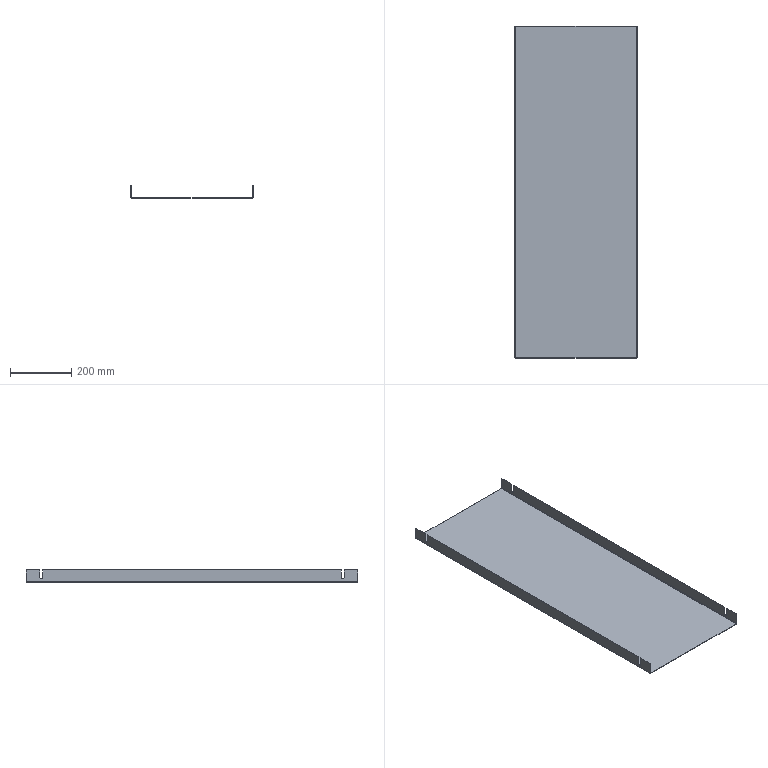Part | STEP file | 1.6米Belt线支撑(Default) | 1 solid | 42 faces | box 400 x 1085 x 40 mm | volume 772332 mm3 | plane 30 | cylinder 12 | commonest cylinder face diameters 9 x8 2 x2 5 x2
STEP:
#1=CARTESIAN_POINT('',(398.5,50.,-29.5));
#2=VERTEX_POINT('',#1);
#3=CARTESIAN_POINT('',(398.5,54.5,-25.));
#4=VERTEX_POINT('',#3);
#5=CARTESIAN_POINT('',(398.5,50.,-25.));
#6=DIRECTION('',(1.,0.,0.));
#7=DIRECTION('',(0.,0.,-1.));
#8=AXIS2_PLACEMENT_3D('',#5,#6,#7);
#9=CIRCLE('',#8,4.5);
#10=EDGE_CURVE('',#2,#4,#9,.T.);
#11=ORIENTED_EDGE('',*,*,#10,.F.);
#12=CARTESIAN_POINT('',(400.,50.,-29.5));
#13=VERTEX_POINT('',#12);
#14=CARTESIAN_POINT('',(0.,50.,-29.5));
#15=DIRECTION('',(1.,0.,0.));
#16=VECTOR('',#15,1000.);
#17=LINE('',#14,#16);
#18=EDGE_CURVE('',#2,#13,#17,.T.);
#19=ORIENTED_EDGE('',*,*,#18,.T.);
#20=CARTESIAN_POINT('',(400.,54.5,-25.));
#21=VERTEX_POINT('',#20);
#22=CARTESIAN_POINT('',(400.,50.,-25.));
#23=DIRECTION('',(1.,0.,0.));
#24=DIRECTION('',(0.,0.,-1.));
#25=AXIS2_PLACEMENT_3D('',#22,#23,#24);
#26=CIRCLE('',#25,4.5);
#27=EDGE_CURVE('',#13,#21,#26,.T.);
#28=ORIENTED_EDGE('',*,*,#27,.T.);
#29=CARTESIAN_POINT('',(0.,54.5,-25.));
#30=DIRECTION('',(1.,0.,0.));
#31=VECTOR('',#30,1000.);
#32=LINE('',#29,#31);
#33=EDGE_CURVE('',#4,#21,#32,.T.);
#34=ORIENTED_EDGE('',*,*,#33,.F.);
#35=EDGE_LOOP('',(#11,#19,#28,#34));
#36=FACE_OUTER_BOUND('',#35,.T.);
#37=CARTESIAN_POINT('',(0.,50.,-25.));
#38=DIRECTION('',(1.,0.,0.));
#39=DIRECTION('',(0.,0.,-1.));
#40=AXIS2_PLACEMENT_3D('',#37,#38,#39);
#41=CYLINDRICAL_SURFACE('',#40,4.5);
#42=ADVANCED_FACE('',(#36),#41,.F.);
#43=CARTESIAN_POINT('',(0.,50.,-29.5));
#44=VERTEX_POINT('',#43);
#45=CARTESIAN_POINT('',(0.,54.5,-25.));
#46=VERTEX_POINT('',#45);
#47=CARTESIAN_POINT('',(0.,50.,-25.));
#48=DIRECTION('',(1.,0.,0.));
#49=DIRECTION('',(0.,0.,-1.));
#50=AXIS2_PLACEMENT_3D('',#47,#48,#49);
#51=CIRCLE('',#50,4.5);
#52=EDGE_CURVE('',#44,#46,#51,.T.);
#53=ORIENTED_EDGE('',*,*,#52,.F.);
#54=CARTESIAN_POINT('',(1.5,50.,-29.5));
#55=VERTEX_POINT('',#54);
#56=CARTESIAN_POINT('',(0.,50.,-29.5));
#57=DIRECTION('',(1.,0.,0.));
#58=VECTOR('',#57,1000.);
#59=LINE('',#56,#58);
#60=EDGE_CURVE('',#44,#55,#59,.T.);
#61=ORIENTED_EDGE('',*,*,#60,.T.);
#62=CARTESIAN_POINT('',(1.5,54.5,-25.));
#63=VERTEX_POINT('',#62);
#64=CARTESIAN_POINT('',(1.5,50.,-25.));
#65=DIRECTION('',(-1.,0.,0.));
#66=DIRECTION('',(0.,0.,1.));
#67=AXIS2_PLACEMENT_3D('',#64,#65,#66);
#68=CIRCLE('',#67,4.5);
#69=EDGE_CURVE('',#63,#55,#68,.T.);
#70=ORIENTED_EDGE('',*,*,#69,.F.);
#71=CARTESIAN_POINT('',(0.,54.5,-25.));
#72=DIRECTION('',(1.,0.,0.));
#73=VECTOR('',#72,1000.);
#74=LINE('',#71,#73);
#75=EDGE_CURVE('',#46,#63,#74,.T.);
#76=ORIENTED_EDGE('',*,*,#75,.F.);
#77=EDGE_LOOP('',(#53,#61,#70,#76));
#78=FACE_OUTER_BOUND('',#77,.T.);
#79=CARTESIAN_POINT('',(0.,50.,-25.));
#80=DIRECTION('',(1.,0.,0.));
#81=DIRECTION('',(0.,0.,-1.));
#82=AXIS2_PLACEMENT_3D('',#79,#80,#81);
#83=CYLINDRICAL_SURFACE('',#82,4.5);
#84=ADVANCED_FACE('',(#78),#83,.F.);
#85=CARTESIAN_POINT('',(398.5,1035.,-29.5));
#86=VERTEX_POINT('',#85);
#87=CARTESIAN_POINT('',(398.5,1039.5,-25.));
#88=VERTEX_POINT('',#87);
#89=CARTESIAN_POINT('',(398.5,1035.,-25.));
#90=DIRECTION('',(1.,0.,0.));
#91=DIRECTION('',(0.,0.,-1.));
#92=AXIS2_PLACEMENT_3D('',#89,#90,#91);
#93=CIRCLE('',#92,4.5);
#94=EDGE_CURVE('',#86,#88,#93,.T.);
#95=ORIENTED_EDGE('',*,*,#94,.F.);
#96=CARTESIAN_POINT('',(400.,1035.,-29.5));
#97=VERTEX_POINT('',#96);
#98=CARTESIAN_POINT('',(0.,1035.,-29.5));
#99=DIRECTION('',(1.,0.,0.));
#100=VECTOR('',#99,1000.);
#101=LINE('',#98,#100);
#102=EDGE_CURVE('',#86,#97,#101,.T.);
#103=ORIENTED_EDGE('',*,*,#102,.T.);
#104=CARTESIAN_POINT('',(400.,1039.5,-25.));
#105=VERTEX_POINT('',#104);
#106=CARTESIAN_POINT('',(400.,1035.,-25.));
#107=DIRECTION('',(1.,0.,0.));
#108=DIRECTION('',(0.,0.,1.));
#109=AXIS2_PLACEMENT_3D('',#106,#107,#108);
#110=CIRCLE('',#109,4.5);
#111=EDGE_CURVE('',#97,#105,#110,.T.);
#112=ORIENTED_EDGE('',*,*,#111,.T.);
#113=CARTESIAN_POINT('',(0.,1039.5,-25.));
#114=DIRECTION('',(1.,0.,0.));
#115=VECTOR('',#114,1000.);
#116=LINE('',#113,#115);
#117=EDGE_CURVE('',#88,#105,#116,.T.);
#118=ORIENTED_EDGE('',*,*,#117,.F.);
#119=EDGE_LOOP('',(#95,#103,#112,#118));
#120=FACE_OUTER_BOUND('',#119,.T.);
#121=CARTESIAN_POINT('',(0.,1035.,-25.));
#122=DIRECTION('',(1.,0.,0.));
#123=DIRECTION('',(0.,0.,-1.));
#124=AXIS2_PLACEMENT_3D('',#121,#122,#123);
#125=CYLINDRICAL_SURFACE('',#124,4.5);
#126=ADVANCED_FACE('',(#120),#125,.F.);
#127=CARTESIAN_POINT('',(0.,1035.,-29.5));
#128=VERTEX_POINT('',#127);
#129=CARTESIAN_POINT('',(0.,1039.5,-25.));
#130=VERTEX_POINT('',#129);
#131=CARTESIAN_POINT('',(0.,1035.,-25.));
#132=DIRECTION('',(1.,0.,0.));
#133=DIRECTION('',(0.,0.,1.));
#134=AXIS2_PLACEMENT_3D('',#131,#132,#133);
#135=CIRCLE('',#134,4.5);
#136=EDGE_CURVE('',#128,#130,#135,.T.);
#137=ORIENTED_EDGE('',*,*,#136,.F.);
#138=CARTESIAN_POINT('',(1.5,1035.,-29.5));
#139=VERTEX_POINT('',#138);
#140=CARTESIAN_POINT('',(0.,1035.,-29.5));
#141=DIRECTION('',(1.,0.,0.));
#142=VECTOR('',#141,1000.);
#143=LINE('',#140,#142);
#144=EDGE_CURVE('',#128,#139,#143,.T.);
#145=ORIENTED_EDGE('',*,*,#144,.T.);
#146=CARTESIAN_POINT('',(1.5,1039.5,-25.));
#147=VERTEX_POINT('',#146);
#148=CARTESIAN_POINT('',(1.5,1035.,-25.));
#149=DIRECTION('',(-1.,0.,0.));
#150=DIRECTION('',(0.,0.,1.));
#151=AXIS2_PLACEMENT_3D('',#148,#149,#150);
#152=CIRCLE('',#151,4.5);
#153=EDGE_CURVE('',#147,#139,#152,.T.);
#154=ORIENTED_EDGE('',*,*,#153,.F.);
#155=CARTESIAN_POINT('',(0.,1039.5,-25.));
#156=DIRECTION('',(1.,0.,0.));
#157=VECTOR('',#156,1000.);
#158=LINE('',#155,#157);
#159=EDGE_CURVE('',#130,#147,#158,.T.);
#160=ORIENTED_EDGE('',*,*,#159,.F.);
#161=EDGE_LOOP('',(#137,#145,#154,#160));
#162=FACE_OUTER_BOUND('',#161,.T.);
#163=CARTESIAN_POINT('',(0.,1035.,-25.));
#164=DIRECTION('',(1.,0.,0.));
#165=DIRECTION('',(0.,0.,-1.));
#166=AXIS2_PLACEMENT_3D('',#163,#164,#165);
#167=CYLINDRICAL_SURFACE('',#166,4.5);
#168=ADVANCED_FACE('',(#162),#167,.F.);
#169=CARTESIAN_POINT('',(398.5,45.5,0.));
#170=VERTEX_POINT('',#169);
#171=CARTESIAN_POINT('',(400.,45.5,0.));
#172=VERTEX_POINT('',#171);
#173=CARTESIAN_POINT('',(400.,45.5,0.));
#174=DIRECTION('',(1.,0.,0.));
#175=VECTOR('',#174,1000.);
#176=LINE('',#173,#175);
#177=EDGE_CURVE('',#170,#172,#176,.T.);
#178=ORIENTED_EDGE('',*,*,#177,.F.);
#179=CARTESIAN_POINT('',(398.5,0.,0.));
#180=VERTEX_POINT('',#179);
#181=CARTESIAN_POINT('',(398.5,1085.,0.));
#182=DIRECTION('',(0.,-1.,0.));
#183=VECTOR('',#182,1000.);
#184=LINE('',#181,#183);
#185=EDGE_CURVE('',#170,#180,#184,.T.);
#186=ORIENTED_EDGE('',*,*,#185,.T.);
#187=CARTESIAN_POINT('',(400.,0.,0.));
#188=VERTEX_POINT('',#187);
#189=CARTESIAN_POINT('',(400.,0.,0.));
#190=DIRECTION('',(-1.,0.,0.));
#191=VECTOR('',#190,1000.);
#192=LINE('',#189,#191);
#193=EDGE_CURVE('',#188,#180,#192,.T.);
#194=ORIENTED_EDGE('',*,*,#193,.F.);
#195=CARTESIAN_POINT('',(400.,1085.,0.));
#196=DIRECTION('',(0.,-1.,0.));
#197=VECTOR('',#196,1000.);
#198=LINE('',#195,#197);
#199=EDGE_CURVE('',#172,#188,#198,.T.);
#200=ORIENTED_EDGE('',*,*,#199,.F.);
#201=EDGE_LOOP('',(#178,#186,#194,#200));
#202=FACE_OUTER_BOUND('',#201,.T.);
#203=CARTESIAN_POINT('',(400.,1085.,0.));
#204=DIRECTION('',(0.,0.,1.));
#205=DIRECTION('',(1.,0.,0.));
#206=AXIS2_PLACEMENT_3D('',#203,#204,#205);
#207=PLANE('',#206);
#208=ADVANCED_FACE('',(#202),#207,.T.);
#209=CARTESIAN_POINT('',(0.,45.5,0.));
#210=VERTEX_POINT('',#209);
#211=CARTESIAN_POINT('',(1.5,45.5,0.));
#212=VERTEX_POINT('',#211);
#213=CARTESIAN_POINT('',(1.5,45.5,0.));
#214=DIRECTION('',(1.,0.,0.));
#215=VECTOR('',#214,1000.);
#216=LINE('',#213,#215);
#217=EDGE_CURVE('',#210,#212,#216,.T.);
#218=ORIENTED_EDGE('',*,*,#217,.F.);
#219=CARTESIAN_POINT('',(0.,0.,0.));
#220=VERTEX_POINT('',#219);
#221=CARTESIAN_POINT('',(0.,1085.,0.));
#222=DIRECTION('',(0.,-1.,0.));
#223=VECTOR('',#222,1000.);
#224=LINE('',#221,#223);
#225=EDGE_CURVE('',#210,#220,#224,.T.);
#226=ORIENTED_EDGE('',*,*,#225,.T.);
#227=CARTESIAN_POINT('',(1.5,0.,0.));
#228=VERTEX_POINT('',#227);
#229=CARTESIAN_POINT('',(1.5,0.,0.));
#230=DIRECTION('',(-1.,0.,0.));
#231=VECTOR('',#230,1000.);
#232=LINE('',#229,#231);
#233=EDGE_CURVE('',#228,#220,#232,.T.);
#234=ORIENTED_EDGE('',*,*,#233,.F.);
#235=CARTESIAN_POINT('',(1.5,1085.,0.));
#236=DIRECTION('',(0.,-1.,0.));
#237=VECTOR('',#236,1000.);
#238=LINE('',#235,#237);
#239=EDGE_CURVE('',#212,#228,#238,.T.);
#240=ORIENTED_EDGE('',*,*,#239,.F.);
#241=EDGE_LOOP('',(#218,#226,#234,#240));
#242=FACE_OUTER_BOUND('',#241,.T.);
#243=CARTESIAN_POINT('',(1.5,1085.,0.));
#244=DIRECTION('',(0.,0.,1.));
#245=DIRECTION('',(1.,0.,0.));
#246=AXIS2_PLACEMENT_3D('',#243,#244,#245);
#247=PLANE('',#246);
#248=ADVANCED_FACE('',(#242),#247,.T.);
#249=CARTESIAN_POINT('',(400.,54.5,0.));
#250=VERTEX_POINT('',#249);
#251=CARTESIAN_POINT('',(398.5,54.5,0.));
#252=VERTEX_POINT('',#251);
#253=CARTESIAN_POINT('',(400.,54.5,0.));
#254=DIRECTION('',(-1.,0.,0.));
#255=VECTOR('',#254,1000.);
#256=LINE('',#253,#255);
#257=EDGE_CURVE('',#250,#252,#256,.T.);
#258=ORIENTED_EDGE('',*,*,#257,.F.);
#259=CARTESIAN_POINT('',(400.,1030.5,0.));
#260=VERTEX_POINT('',#259);
#261=CARTESIAN_POINT('',(400.,1085.,0.));
#262=DIRECTION('',(0.,-1.,0.));
#263=VECTOR('',#262,1000.);
#264=LINE('',#261,#263);
#265=EDGE_CURVE('',#260,#250,#264,.T.);
#266=ORIENTED_EDGE('',*,*,#265,.F.);
#267=CARTESIAN_POINT('',(398.5,1030.5,0.));
#268=VERTEX_POINT('',#267);
#269=CARTESIAN_POINT('',(400.,1030.5,0.));
#270=DIRECTION('',(1.,0.,0.));
#271=VECTOR('',#270,1000.);
#272=LINE('',#269,#271);
#273=EDGE_CURVE('',#268,#260,#272,.T.);
#274=ORIENTED_EDGE('',*,*,#273,.F.);
#275=CARTESIAN_POINT('',(398.5,1085.,0.));
#276=DIRECTION('',(0.,-1.,0.));
#277=VECTOR('',#276,1000.);
#278=LINE('',#275,#277);
#279=EDGE_CURVE('',#268,#252,#278,.T.);
#280=ORIENTED_EDGE('',*,*,#279,.T.);
#281=EDGE_LOOP('',(#258,#266,#274,#280));
#282=FACE_OUTER_BOUND('',#281,.T.);
#283=CARTESIAN_POINT('',(400.,1085.,0.));
#284=DIRECTION('',(0.,0.,1.));
#285=DIRECTION('',(1.,0.,0.));
#286=AXIS2_PLACEMENT_3D('',#283,#284,#285);
#287=PLANE('',#286);
#288=ADVANCED_FACE('',(#282),#287,.T.);
#289=CARTESIAN_POINT('',(1.5,54.5,0.));
#290=VERTEX_POINT('',#289);
#291=CARTESIAN_POINT('',(0.,54.5,0.));
#292=VERTEX_POINT('',#291);
#293=CARTESIAN_POINT('',(1.5,54.5,0.));
#294=DIRECTION('',(-1.,0.,0.));
#295=VECTOR('',#294,1000.);
#296=LINE('',#293,#295);
#297=EDGE_CURVE('',#290,#292,#296,.T.);
#298=ORIENTED_EDGE('',*,*,#297,.F.);
#299=CARTESIAN_POINT('',(1.5,1030.5,0.));
#300=VERTEX_POINT('',#299);
#301=CARTESIAN_POINT('',(1.5,1085.,0.));
#302=DIRECTION('',(0.,-1.,0.));
#303=VECTOR('',#302,1000.);
#304=LINE('',#301,#303);
#305=EDGE_CURVE('',#300,#290,#304,.T.);
#306=ORIENTED_EDGE('',*,*,#305,.F.);
#307=CARTESIAN_POINT('',(0.,1030.5,0.));
#308=VERTEX_POINT('',#307);
#309=CARTESIAN_POINT('',(1.5,1030.5,0.));
#310=DIRECTION('',(1.,0.,0.));
#311=VECTOR('',#310,1000.);
#312=LINE('',#309,#311);
#313=EDGE_CURVE('',#308,#300,#312,.T.);
#314=ORIENTED_EDGE('',*,*,#313,.F.);
#315=CARTESIAN_POINT('',(0.,1085.,0.));
#316=DIRECTION('',(0.,-1.,0.));
#317=VECTOR('',#316,1000.);
#318=LINE('',#315,#317);
#319=EDGE_CURVE('',#308,#292,#318,.T.);
#320=ORIENTED_EDGE('',*,*,#319,.T.);
#321=EDGE_LOOP('',(#298,#306,#314,#320));
#322=FACE_OUTER_BOUND('',#321,.T.);
#323=CARTESIAN_POINT('',(1.5,1085.,0.));
#324=DIRECTION('',(0.,0.,1.));
#325=DIRECTION('',(1.,0.,0.));
#326=AXIS2_PLACEMENT_3D('',#323,#324,#325);
#327=PLANE('',#326);
#328=ADVANCED_FACE('',(#322),#327,.T.);
#329=CARTESIAN_POINT('',(2.5,1085.,-40.));
#330=VERTEX_POINT('',#329);
#331=CARTESIAN_POINT('',(2.5,1085.,-38.5));
#332=VERTEX_POINT('',#331);
#333=CARTESIAN_POINT('',(2.5,1085.,-40.));
#334=DIRECTION('',(0.,0.,1.));
#335=VECTOR('',#334,1000.);
#336=LINE('',#333,#335);
#337=EDGE_CURVE('',#330,#332,#336,.T.);
#338=ORIENTED_EDGE('',*,*,#337,.F.);
#339=CARTESIAN_POINT('',(0.,1085.,-37.5));
#340=VERTEX_POINT('',#339);
#341=CARTESIAN_POINT('',(2.5,1085.,-37.5));
#342=DIRECTION('',(0.,-1.,0.));
#343=DIRECTION('',(0.,0.,1.));
#344=AXIS2_PLACEMENT_3D('',#341,#342,#343);
#345=CIRCLE('',#344,2.5);
#346=EDGE_CURVE('',#340,#330,#345,.T.);
#347=ORIENTED_EDGE('',*,*,#346,.F.);
#348=CARTESIAN_POINT('',(1.5,1085.,-37.5));
#349=VERTEX_POINT('',#348);
#350=CARTESIAN_POINT('',(1.5,1085.,-37.5));
#351=DIRECTION('',(-1.,0.,0.));
#352=VECTOR('',#351,1000.);
#353=LINE('',#350,#352);
#354=EDGE_CURVE('',#349,#340,#353,.T.);
#355=ORIENTED_EDGE('',*,*,#354,.F.);
#356=CARTESIAN_POINT('',(2.5,1085.,-37.5));
#357=DIRECTION('',(0.,-1.,0.));
#358=DIRECTION('',(1.,0.,0.));
#359=AXIS2_PLACEMENT_3D('',#356,#357,#358);
#360=CIRCLE('',#359,1.);
#361=EDGE_CURVE('',#349,#332,#360,.T.);
#362=ORIENTED_EDGE('',*,*,#361,.T.);
#363=EDGE_LOOP('',(#338,#347,#355,#362));
#364=FACE_OUTER_BOUND('',#363,.T.);
#365=CARTESIAN_POINT('',(2.5,1085.,-40.));
#366=DIRECTION('',(0.,1.,0.));
#367=DIRECTION('',(0.,0.,1.));
#368=AXIS2_PLACEMENT_3D('',#365,#366,#367);
#369=PLANE('',#368);
#370=ADVANCED_FACE('',(#364),#369,.T.);
#371=CARTESIAN_POINT('',(397.5,1085.,-40.));
#372=VERTEX_POINT('',#371);
#373=CARTESIAN_POINT('',(0.,1085.,-40.));
#374=DIRECTION('',(1.,0.,0.));
#375=VECTOR('',#374,1000.);
#376=LINE('',#373,#375);
#377=EDGE_CURVE('',#330,#372,#376,.T.);
#378=ORIENTED_EDGE('',*,*,#377,.F.);
#379=ORIENTED_EDGE('',*,*,#337,.T.);
#380=CARTESIAN_POINT('',(397.5,1085.,-38.5));
#381=VERTEX_POINT('',#380);
#382=CARTESIAN_POINT('',(0.,1085.,-38.5));
#383=DIRECTION('',(1.,0.,0.));
#384=VECTOR('',#383,1000.);
#385=LINE('',#382,#384);
#386=EDGE_CURVE('',#332,#381,#385,.T.);
#387=ORIENTED_EDGE('',*,*,#386,.T.);
#388=CARTESIAN_POINT('',(397.5,1085.,-38.5));
#389=DIRECTION('',(0.,0.,-1.));
#390=VECTOR('',#389,1000.);
#391=LINE('',#388,#390);
#392=EDGE_CURVE('',#381,#372,#391,.T.);
#393=ORIENTED_EDGE('',*,*,#392,.T.);
#394=EDGE_LOOP('',(#378,#379,#387,#393));
#395=FACE_OUTER_BOUND('',#394,.T.);
#396=CARTESIAN_POINT('',(1.5,1085.,-37.5));
#397=DIRECTION('',(0.,1.,0.));
#398=DIRECTION('',(0.,0.,1.));
#399=AXIS2_PLACEMENT_3D('',#396,#397,#398);
#400=PLANE('',#399);
#401=ADVANCED_FACE('',(#395),#400,.T.);
#402=CARTESIAN_POINT('',(0.,0.,-37.5));
#403=VERTEX_POINT('',#402);
#404=CARTESIAN_POINT('',(1.5,0.,-37.5));
#405=VERTEX_POINT('',#404);
#406=CARTESIAN_POINT('',(0.,0.,-37.5));
#407=DIRECTION('',(1.,0.,0.));
#408=VECTOR('',#407,1000.);
#409=LINE('',#406,#408);
#410=EDGE_CURVE('',#403,#405,#409,.T.);
#411=ORIENTED_EDGE('',*,*,#410,.F.);
#412=CARTESIAN_POINT('',(2.5,0.,-40.));
#413=VERTEX_POINT('',#412);
#414=CARTESIAN_POINT('',(2.5,0.,-37.5));
#415=DIRECTION('',(0.,-1.,0.));
#416=DIRECTION('',(0.,0.,1.));
#417=AXIS2_PLACEMENT_3D('',#414,#415,#416);
#418=CIRCLE('',#417,2.5);
#419=EDGE_CURVE('',#403,#413,#418,.T.);
#420=ORIENTED_EDGE('',*,*,#419,.T.);
#421=CARTESIAN_POINT('',(2.5,0.,-38.5));
#422=VERTEX_POINT('',#421);
#423=CARTESIAN_POINT('',(2.5,0.,-38.5));
#424=DIRECTION('',(0.,0.,-1.));
#425=VECTOR('',#424,1000.);
#426=LINE('',#423,#425);
#427=EDGE_CURVE('',#422,#413,#426,.T.);
#428=ORIENTED_EDGE('',*,*,#427,.F.);
#429=CARTESIAN_POINT('',(2.5,0.,-37.5));
#430=DIRECTION('',(0.,-1.,0.));
#431=DIRECTION('',(1.,0.,0.));
#432=AXIS2_PLACEMENT_3D('',#429,#430,#431);
#433=CIRCLE('',#432,1.);
#434=EDGE_CURVE('',#405,#422,#433,.T.);
#435=ORIENTED_EDGE('',*,*,#434,.F.);
#436=EDGE_LOOP('',(#411,#420,#428,#435));
#437=FACE_OUTER_BOUND('',#436,.T.);
#438=CARTESIAN_POINT('',(0.,0.,-37.5));
#439=DIRECTION('',(0.,-1.,0.));
#440=DIRECTION('',(0.,0.,-1.));
#441=AXIS2_PLACEMENT_3D('',#438,#439,#440);
#442=PLANE('',#441);
#443=ADVANCED_FACE('',(#437),#442,.T.);
#444=CARTESIAN_POINT('',(0.,0.,0.));
#445=DIRECTION('',(0.,0.,-1.));
#446=VECTOR('',#445,1000.);
#447=LINE('',#444,#446);
#448=EDGE_CURVE('',#220,#403,#447,.T.);
#449=ORIENTED_EDGE('',*,*,#448,.T.);
#450=ORIENTED_EDGE('',*,*,#410,.T.);
#451=CARTESIAN_POINT('',(1.5,0.,0.));
#452=DIRECTION('',(0.,0.,-1.));
#453=VECTOR('',#452,1000.);
#454=LINE('',#451,#453);
#455=EDGE_CURVE('',#228,#405,#454,.T.);
#456=ORIENTED_EDGE('',*,*,#455,.F.);
#457=ORIENTED_EDGE('',*,*,#233,.T.);
#458=EDGE_LOOP('',(#449,#450,#456,#457));
#459=FACE_OUTER_BOUND('',#458,.T.);
#460=CARTESIAN_POINT('',(2.5,0.,-38.5));
#461=DIRECTION('',(0.,-1.,0.));
#462=DIRECTION('',(0.,0.,-1.));
#463=AXIS2_PLACEMENT_3D('',#460,#461,#462);
#464=PLANE('',#463);
#465=ADVANCED_FACE('',(#459),#464,.T.);
#466=CARTESIAN_POINT('',(400.,1085.,-37.5));
#467=VERTEX_POINT('',#466);
#468=CARTESIAN_POINT('',(398.5,1085.,-37.5));
#469=VERTEX_POINT('',#468);
#470=CARTESIAN_POINT('',(400.,1085.,-37.5));
#471=DIRECTION('',(-1.,0.,0.));
#472=VECTOR('',#471,1000.);
#473=LINE('',#470,#472);
#474=EDGE_CURVE('',#467,#469,#473,.T.);
#475=ORIENTED_EDGE('',*,*,#474,.F.);
#476=CARTESIAN_POINT('',(397.5,1085.,-37.5));
#477=DIRECTION('',(0.,-1.,0.));
#478=DIRECTION('',(0.,0.,1.));
#479=AXIS2_PLACEMENT_3D('',#476,#477,#478);
#480=CIRCLE('',#479,2.5);
#481=EDGE_CURVE('',#372,#467,#480,.T.);
#482=ORIENTED_EDGE('',*,*,#481,.F.);
#483=ORIENTED_EDGE('',*,*,#392,.F.);
#484=CARTESIAN_POINT('',(397.5,1085.,-37.5));
#485=DIRECTION('',(0.,-1.,0.));
#486=DIRECTION('',(1.,0.,0.));
#487=AXIS2_PLACEMENT_3D('',#484,#485,#486);
#488=CIRCLE('',#487,1.);
#489=EDGE_CURVE('',#381,#469,#488,.T.);
#490=ORIENTED_EDGE('',*,*,#489,.T.);
#491=EDGE_LOOP('',(#475,#482,#483,#490));
#492=FACE_OUTER_BOUND('',#491,.T.);
#493=CARTESIAN_POINT('',(400.,1085.,-37.5));
#494=DIRECTION('',(0.,1.,0.));
#495=DIRECTION('',(0.,0.,1.));
#496=AXIS2_PLACEMENT_3D('',#493,#494,#495);
#497=PLANE('',#496);
#498=ADVANCED_FACE('',(#492),#497,.T.);
#499=CARTESIAN_POINT('',(400.,1085.,0.));
#500=VERTEX_POINT('',#499);
#501=CARTESIAN_POINT('',(400.,1085.,-40.));
#502=DIRECTION('',(0.,0.,1.));
#503=VECTOR('',#502,1000.);
#504=LINE('',#501,#503);
#505=EDGE_CURVE('',#467,#500,#504,.T.);
#506=ORIENTED_EDGE('',*,*,#505,.F.);
#507=ORIENTED_EDGE('',*,*,#474,.T.);
#508=CARTESIAN_POINT('',(398.5,1085.,0.));
#509=VERTEX_POINT('',#508);
#510=CARTESIAN_POINT('',(398.5,1085.,-40.));
#511=DIRECTION('',(0.,0.,1.));
#512=VECTOR('',#511,1000.);
#513=LINE('',#510,#512);
#514=EDGE_CURVE('',#469,#509,#513,.T.);
#515=ORIENTED_EDGE('',*,*,#514,.T.);
#516=CARTESIAN_POINT('',(400.,1085.,0.));
#517=DIRECTION('',(-1.,0.,0.));
#518=VECTOR('',#517,1000.);
#519=LINE('',#516,#518);
#520=EDGE_CURVE('',#500,#509,#519,.T.);
#521=ORIENTED_EDGE('',*,*,#520,.F.);
#522=EDGE_LOOP('',(#506,#507,#515,#521));
#523=FACE_OUTER_BOUND('',#522,.T.);
#524=CARTESIAN_POINT('',(397.5,1085.,-38.5));
#525=DIRECTION('',(0.,1.,0.));
#526=DIRECTION('',(0.,0.,1.));
#527=AXIS2_PLACEMENT_3D('',#524,#525,#526);
#528=PLANE('',#527);
#529=ADVANCED_FACE('',(#523),#528,.T.);
#530=CARTESIAN_POINT('',(397.5,0.,-40.));
#531=VERTEX_POINT('',#530);
#532=CARTESIAN_POINT('',(397.5,0.,-38.5));
#533=VERTEX_POINT('',#532);
#534=CARTESIAN_POINT('',(397.5,0.,-40.));
#535=DIRECTION('',(0.,0.,1.));
#536=VECTOR('',#535,1000.);
#537=LINE('',#534,#536);
#538=EDGE_CURVE('',#531,#533,#537,.T.);
#539=ORIENTED_EDGE('',*,*,#538,.F.);
#540=CARTESIAN_POINT('',(400.,0.,-37.5));
#541=VERTEX_POINT('',#540);
#542=CARTESIAN_POINT('',(397.5,0.,-37.5));
#543=DIRECTION('',(0.,-1.,0.));
#544=DIRECTION('',(0.,0.,1.));
#545=AXIS2_PLACEMENT_3D('',#542,#543,#544);
#546=CIRCLE('',#545,2.5);
#547=EDGE_CURVE('',#531,#541,#546,.T.);
#548=ORIENTED_EDGE('',*,*,#547,.T.);
#549=CARTESIAN_POINT('',(398.5,0.,-37.5));
#550=VERTEX_POINT('',#549);
#551=CARTESIAN_POINT('',(398.5,0.,-37.5));
#552=DIRECTION('',(1.,0.,0.));
#553=VECTOR('',#552,1000.);
#554=LINE('',#551,#553);
#555=EDGE_CURVE('',#550,#541,#554,.T.);
#556=ORIENTED_EDGE('',*,*,#555,.F.);
#557=CARTESIAN_POINT('',(397.5,0.,-37.5));
#558=DIRECTION('',(0.,-1.,0.));
#559=DIRECTION('',(1.,0.,0.));
#560=AXIS2_PLACEMENT_3D('',#557,#558,#559);
#561=CIRCLE('',#560,1.);
#562=EDGE_CURVE('',#533,#550,#561,.T.);
#563=ORIENTED_EDGE('',*,*,#562,.F.);
#564=EDGE_LOOP('',(#539,#548,#556,#563));
#565=FACE_OUTER_BOUND('',#564,.T.);
#566=CARTESIAN_POINT('',(397.5,0.,-40.));
#567=DIRECTION('',(0.,-1.,0.));
#568=DIRECTION('',(0.,0.,-1.));
#569=AXIS2_PLACEMENT_3D('',#566,#567,#568);
#570=PLANE('',#569);
#571=ADVANCED_FACE('',(#565),#570,.T.);
#572=CARTESIAN_POINT('',(0.,0.,-40.));
#573=DIRECTION('',(1.,0.,0.));
#574=VECTOR('',#573,1000.);
#575=LINE('',#572,#574);
#576=EDGE_CURVE('',#413,#531,#575,.T.);
#577=ORIENTED_EDGE('',*,*,#576,.T.);
#578=ORIENTED_EDGE('',*,*,#538,.T.);
#579=CARTESIAN_POINT('',(0.,0.,-38.5));
#580=DIRECTION('',(1.,0.,0.));
#581=VECTOR('',#580,1000.);
#582=LINE('',#579,#581);
#583=EDGE_CURVE('',#422,#533,#582,.T.);
#584=ORIENTED_EDGE('',*,*,#583,.F.);
#585=ORIENTED_EDGE('',*,*,#427,.T.);
#586=EDGE_LOOP('',(#577,#578,#584,#585));
#587=FACE_OUTER_BOUND('',#586,.T.);
#588=CARTESIAN_POINT('',(398.5,0.,-37.5));
#589=DIRECTION('',(0.,-1.,0.));
#590=DIRECTION('',(0.,0.,-1.));
#591=AXIS2_PLACEMENT_3D('',#588,#589,#590);
#592=PLANE('',#591);
#593=ADVANCED_FACE('',(#587),#592,.T.);
#594=ORIENTED_EDGE('',*,*,#185,.F.);
#595=CARTESIAN_POINT('',(398.5,45.5,-25.));
#596=VERTEX_POINT('',#595);
#597=CARTESIAN_POINT('',(398.5,45.5,-40.));
#598=DIRECTION('',(0.,0.,-1.));
#599=VECTOR('',#598,1000.);
#600=LINE('',#597,#599);
#601=EDGE_CURVE('',#170,#596,#600,.T.);
#602=ORIENTED_EDGE('',*,*,#601,.T.);
#603=CARTESIAN_POINT('',(398.5,50.,-25.));
#604=DIRECTION('',(1.,0.,0.));
#605=DIRECTION('',(0.,0.,-1.));
#606=AXIS2_PLACEMENT_3D('',#603,#604,#605);
#607=CIRCLE('',#606,4.5);
#608=EDGE_CURVE('',#596,#2,#607,.T.);
#609=ORIENTED_EDGE('',*,*,#608,.T.);
#610=ORIENTED_EDGE('',*,*,#10,.T.);
#611=CARTESIAN_POINT('',(398.5,54.5,-40.));
#612=DIRECTION('',(0.,0.,1.));
#613=VECTOR('',#612,1000.);
#614=LINE('',#611,#613);
#615=EDGE_CURVE('',#4,#252,#614,.T.);
#616=ORIENTED_EDGE('',*,*,#615,.T.);
#617=ORIENTED_EDGE('',*,*,#279,.F.);
#618=CARTESIAN_POINT('',(398.5,1030.5,-25.));
#619=VERTEX_POINT('',#618);
#620=CARTESIAN_POINT('',(398.5,1030.5,-40.));
#621=DIRECTION('',(0.,0.,-1.));
#622=VECTOR('',#621,1000.);
#623=LINE('',#620,#622);
#624=EDGE_CURVE('',#268,#619,#623,.T.);
#625=ORIENTED_EDGE('',*,*,#624,.T.);
#626=CARTESIAN_POINT('',(398.5,1035.,-25.));
#627=DIRECTION('',(1.,0.,0.));
#628=DIRECTION('',(0.,0.,-1.));
#629=AXIS2_PLACEMENT_3D('',#626,#627,#628);
#630=CIRCLE('',#629,4.5);
#631=EDGE_CURVE('',#619,#86,#630,.T.);
#632=ORIENTED_EDGE('',*,*,#631,.T.);
#633=ORIENTED_EDGE('',*,*,#94,.T.);
#634=CARTESIAN_POINT('',(398.5,1039.5,0.));
#635=VERTEX_POINT('',#634);
#636=CARTESIAN_POINT('',(398.5,1039.5,-40.));
#637=DIRECTION('',(0.,0.,1.));
#638=VECTOR('',#637,1000.);
#639=LINE('',#636,#638);
#640=EDGE_CURVE('',#88,#635,#639,.T.);
#641=ORIENTED_EDGE('',*,*,#640,.T.);
#642=CARTESIAN_POINT('',(398.5,1085.,0.));
#643=DIRECTION('',(0.,-1.,0.));
#644=VECTOR('',#643,1000.);
#645=LINE('',#642,#644);
#646=EDGE_CURVE('',#509,#635,#645,.T.);
#647=ORIENTED_EDGE('',*,*,#646,.F.);
#648=ORIENTED_EDGE('',*,*,#514,.F.);
#649=CARTESIAN_POINT('',(398.5,1085.,-37.5));
#650=DIRECTION('',(0.,-1.,0.));
#651=VECTOR('',#650,1000.);
#652=LINE('',#649,#651);
#653=EDGE_CURVE('',#469,#550,#652,.T.);
#654=ORIENTED_EDGE('',*,*,#653,.T.);
#655=CARTESIAN_POINT('',(398.5,0.,-40.));
#656=DIRECTION('',(0.,0.,1.));
#657=VECTOR('',#656,1000.);
#658=LINE('',#655,#657);
#659=EDGE_CURVE('',#550,#180,#658,.T.);
#660=ORIENTED_EDGE('',*,*,#659,.T.);
#661=EDGE_LOOP('',(#594,#602,#609,#610,#616,#617,#625,#632,#633,#641,#647,#648,#654,#660));
#662=FACE_OUTER_BOUND('',#661,.T.);
#663=CARTESIAN_POINT('',(398.5,1085.,-40.));
#664=DIRECTION('',(1.,0.,0.));
#665=DIRECTION('',(0.,0.,-1.));
#666=AXIS2_PLACEMENT_3D('',#663,#664,#665);
#667=PLANE('',#666);
#668=ADVANCED_FACE('',(#662),#667,.F.);
#669=CARTESIAN_POINT('',(400.,1039.5,0.));
#670=VERTEX_POINT('',#669);
#671=CARTESIAN_POINT('',(400.,1039.5,0.));
#672=DIRECTION('',(-1.,0.,0.));
#673=VECTOR('',#672,1000.);
#674=LINE('',#671,#673);
#675=EDGE_CURVE('',#670,#635,#674,.T.);
#676=ORIENTED_EDGE('',*,*,#675,.F.);
#677=CARTESIAN_POINT('',(400.,1085.,0.));
#678=DIRECTION('',(0.,-1.,0.));
#679=VECTOR('',#678,1000.);
#680=LINE('',#677,#679);
#681=EDGE_CURVE('',#500,#670,#680,.T.);
#682=ORIENTED_EDGE('',*,*,#681,.F.);
#683=ORIENTED_EDGE('',*,*,#520,.T.);
#684=ORIENTED_EDGE('',*,*,#646,.T.);
#685=EDGE_LOOP('',(#676,#682,#683,#684));
#686=FACE_OUTER_BOUND('',#685,.T.);
#687=CARTESIAN_POINT('',(400.,1085.,0.));
#688=DIRECTION('',(0.,0.,1.));
#689=DIRECTION('',(1.,0.,0.));
#690=AXIS2_PLACEMENT_3D('',#687,#688,#689);
#691=PLANE('',#690);
#692=ADVANCED_FACE('',(#686),#691,.T.);
#693=CARTESIAN_POINT('',(400.,45.5,-25.));
#694=VERTEX_POINT('',#693);
#695=CARTESIAN_POINT('',(400.,45.5,-25.));
#696=DIRECTION('',(0.,0.,-1.));
#697=VECTOR('',#696,1000.);
#698=LINE('',#695,#697);
#699=EDGE_CURVE('',#172,#694,#698,.T.);
#700=ORIENTED_EDGE('',*,*,#699,.F.);
#701=ORIENTED_EDGE('',*,*,#199,.T.);
#702=CARTESIAN_POINT('',(400.,0.,-40.));
#703=DIRECTION('',(0.,0.,1.));
#704=VECTOR('',#703,1000.);
#705=LINE('',#702,#704);
#706=EDGE_CURVE('',#541,#188,#705,.T.);
#707=ORIENTED_EDGE('',*,*,#706,.F.);
#708=CARTESIAN_POINT('',(400.,1085.,-37.5));
#709=DIRECTION('',(0.,-1.,0.));
#710=VECTOR('',#709,1000.);
#711=LINE('',#708,#710);
#712=EDGE_CURVE('',#467,#541,#711,.T.);
#713=ORIENTED_EDGE('',*,*,#712,.F.);
#714=ORIENTED_EDGE('',*,*,#505,.T.);
#715=ORIENTED_EDGE('',*,*,#681,.T.);
#716=CARTESIAN_POINT('',(400.,1039.5,-25.));
#717=DIRECTION('',(0.,0.,1.));
#718=VECTOR('',#717,1000.);
#719=LINE('',#716,#718);
#720=EDGE_CURVE('',#105,#670,#719,.T.);
#721=ORIENTED_EDGE('',*,*,#720,.F.);
#722=ORIENTED_EDGE('',*,*,#111,.F.);
#723=CARTESIAN_POINT('',(400.,1030.5,-25.));
#724=VERTEX_POINT('',#723);
#725=CARTESIAN_POINT('',(400.,1035.,-25.));
#726=DIRECTION('',(1.,0.,0.));
#727=DIRECTION('',(0.,0.,1.));
#728=AXIS2_PLACEMENT_3D('',#725,#726,#727);
#729=CIRCLE('',#728,4.5);
#730=EDGE_CURVE('',#724,#97,#729,.T.);
#731=ORIENTED_EDGE('',*,*,#730,.F.);
#732=CARTESIAN_POINT('',(400.,1030.5,-25.));
#733=DIRECTION('',(0.,0.,-1.));
#734=VECTOR('',#733,1000.);
#735=LINE('',#732,#734);
#736=EDGE_CURVE('',#260,#724,#735,.T.);
#737=ORIENTED_EDGE('',*,*,#736,.F.);
#738=ORIENTED_EDGE('',*,*,#265,.T.);
#739=CARTESIAN_POINT('',(400.,54.5,-25.));
#740=DIRECTION('',(0.,0.,1.));
#741=VECTOR('',#740,1000.);
#742=LINE('',#739,#741);
#743=EDGE_CURVE('',#21,#250,#742,.T.);
#744=ORIENTED_EDGE('',*,*,#743,.F.);
#745=ORIENTED_EDGE('',*,*,#27,.F.);
#746=CARTESIAN_POINT('',(400.,50.,-25.));
#747=DIRECTION('',(1.,0.,0.));
#748=DIRECTION('',(0.,0.,-1.));
#749=AXIS2_PLACEMENT_3D('',#746,#747,#748);
#750=CIRCLE('',#749,4.5);
#751=EDGE_CURVE('',#694,#13,#750,.T.);
#752=ORIENTED_EDGE('',*,*,#751,.F.);
#753=EDGE_LOOP('',(#700,#701,#707,#713,#714,#715,#721,#722,#731,#737,#738,#744,#745,#752));
#754=FACE_OUTER_BOUND('',#753,.T.);
#755=CARTESIAN_POINT('',(400.,1085.,-40.));
#756=DIRECTION('',(1.,0.,0.));
#757=DIRECTION('',(0.,0.,-1.));
#758=AXIS2_PLACEMENT_3D('',#755,#756,#757);
#759=PLANE('',#758);
#760=ADVANCED_FACE('',(#754),#759,.T.);
#761=ORIENTED_EDGE('',*,*,#547,.F.);
#762=CARTESIAN_POINT('',(397.5,1085.,-40.));
#763=DIRECTION('',(0.,-1.,0.));
#764=VECTOR('',#763,1000.);
#765=LINE('',#762,#764);
#766=EDGE_CURVE('',#372,#531,#765,.T.);
#767=ORIENTED_EDGE('',*,*,#766,.F.);
#768=ORIENTED_EDGE('',*,*,#481,.T.);
#769=ORIENTED_EDGE('',*,*,#712,.T.);
#770=EDGE_LOOP('',(#761,#767,#768,#769));
#771=FACE_OUTER_BOUND('',#770,.T.);
#772=CARTESIAN_POINT('',(397.5,1085.,-37.5));
#773=DIRECTION('',(0.,-1.,0.));
#774=DIRECTION('',(0.,0.,-1.));
#775=AXIS2_PLACEMENT_3D('',#772,#773,#774);
#776=CYLINDRICAL_SURFACE('',#775,2.5);
#777=ADVANCED_FACE('',(#771),#776,.T.);
#778=ORIENTED_EDGE('',*,*,#576,.F.);
#779=CARTESIAN_POINT('',(2.5,1085.,-40.));
#780=DIRECTION('',(0.,-1.,0.));
#781=VECTOR('',#780,1000.);
#782=LINE('',#779,#781);
#783=EDGE_CURVE('',#330,#413,#782,.T.);
#784=ORIENTED_EDGE('',*,*,#783,.F.);
#785=ORIENTED_EDGE('',*,*,#377,.T.);
#786=ORIENTED_EDGE('',*,*,#766,.T.);
#787=EDGE_LOOP('',(#778,#784,#785,#786));
#788=FACE_OUTER_BOUND('',#787,.T.);
#789=CARTESIAN_POINT('',(0.,1085.,-40.));
#790=DIRECTION('',(0.,0.,-1.));
#791=DIRECTION('',(-1.,0.,0.));
#792=AXIS2_PLACEMENT_3D('',#789,#790,#791);
#793=PLANE('',#792);
#794=ADVANCED_FACE('',(#788),#793,.T.);
#795=ORIENTED_EDGE('',*,*,#419,.F.);
#796=CARTESIAN_POINT('',(0.,1085.,-37.5));
#797=DIRECTION('',(0.,-1.,0.));
#798=VECTOR('',#797,1000.);
#799=LINE('',#796,#798);
#800=EDGE_CURVE('',#340,#403,#799,.T.);
#801=ORIENTED_EDGE('',*,*,#800,.F.);
#802=ORIENTED_EDGE('',*,*,#346,.T.);
#803=ORIENTED_EDGE('',*,*,#783,.T.);
#804=EDGE_LOOP('',(#795,#801,#802,#803));
#805=FACE_OUTER_BOUND('',#804,.T.);
#806=CARTESIAN_POINT('',(2.5,1085.,-37.5));
#807=DIRECTION('',(0.,-1.,0.));
#808=DIRECTION('',(0.,0.,-1.));
#809=AXIS2_PLACEMENT_3D('',#806,#807,#808);
#810=CYLINDRICAL_SURFACE('',#809,2.5);
#811=ADVANCED_FACE('',(#805),#810,.T.);
#812=CARTESIAN_POINT('',(0.,45.5,-25.));
#813=VERTEX_POINT('',#812);
#814=CARTESIAN_POINT('',(0.,45.5,-25.));
#815=DIRECTION('',(0.,0.,-1.));
#816=VECTOR('',#815,1000.);
#817=LINE('',#814,#816);
#818=EDGE_CURVE('',#210,#813,#817,.T.);
#819=ORIENTED_EDGE('',*,*,#818,.T.);
#820=CARTESIAN_POINT('',(0.,50.,-25.));
#821=DIRECTION('',(1.,0.,0.));
#822=DIRECTION('',(0.,0.,-1.));
#823=AXIS2_PLACEMENT_3D('',#820,#821,#822);
#824=CIRCLE('',#823,4.5);
#825=EDGE_CURVE('',#813,#44,#824,.T.);
#826=ORIENTED_EDGE('',*,*,#825,.T.);
#827=ORIENTED_EDGE('',*,*,#52,.T.);
#828=CARTESIAN_POINT('',(0.,54.5,-25.));
#829=DIRECTION('',(0.,0.,1.));
#830=VECTOR('',#829,1000.);
#831=LINE('',#828,#830);
#832=EDGE_CURVE('',#46,#292,#831,.T.);
#833=ORIENTED_EDGE('',*,*,#832,.T.);
#834=ORIENTED_EDGE('',*,*,#319,.F.);
#835=CARTESIAN_POINT('',(0.,1030.5,-25.));
#836=VERTEX_POINT('',#835);
#837=CARTESIAN_POINT('',(0.,1030.5,-25.));
#838=DIRECTION('',(0.,0.,-1.));
#839=VECTOR('',#838,1000.);
#840=LINE('',#837,#839);
#841=EDGE_CURVE('',#308,#836,#840,.T.);
#842=ORIENTED_EDGE('',*,*,#841,.T.);
#843=CARTESIAN_POINT('',(0.,1035.,-25.));
#844=DIRECTION('',(1.,0.,0.));
#845=DIRECTION('',(0.,0.,1.));
#846=AXIS2_PLACEMENT_3D('',#843,#844,#845);
#847=CIRCLE('',#846,4.5);
#848=EDGE_CURVE('',#836,#128,#847,.T.);
#849=ORIENTED_EDGE('',*,*,#848,.T.);
#850=ORIENTED_EDGE('',*,*,#136,.T.);
#851=CARTESIAN_POINT('',(0.,1039.5,0.));
#852=VERTEX_POINT('',#851);
#853=CARTESIAN_POINT('',(0.,1039.5,-25.));
#854=DIRECTION('',(0.,0.,1.));
#855=VECTOR('',#854,1000.);
#856=LINE('',#853,#855);
#857=EDGE_CURVE('',#130,#852,#856,.T.);
#858=ORIENTED_EDGE('',*,*,#857,.T.);
#859=CARTESIAN_POINT('',(0.,1085.,0.));
#860=VERTEX_POINT('',#859);
#861=CARTESIAN_POINT('',(0.,1085.,0.));
#862=DIRECTION('',(0.,-1.,0.));
#863=VECTOR('',#862,1000.);
#864=LINE('',#861,#863);
#865=EDGE_CURVE('',#860,#852,#864,.T.);
#866=ORIENTED_EDGE('',*,*,#865,.F.);
#867=CARTESIAN_POINT('',(0.,1085.,0.));
#868=DIRECTION('',(0.,0.,-1.));
#869=VECTOR('',#868,1000.);
#870=LINE('',#867,#869);
#871=EDGE_CURVE('',#860,#340,#870,.T.);
#872=ORIENTED_EDGE('',*,*,#871,.T.);
#873=ORIENTED_EDGE('',*,*,#800,.T.);
#874=ORIENTED_EDGE('',*,*,#448,.F.);
#875=ORIENTED_EDGE('',*,*,#225,.F.);
#876=EDGE_LOOP('',(#819,#826,#827,#833,#834,#842,#849,#850,#858,#866,#872,#873,#874,#875));
#877=FACE_OUTER_BOUND('',#876,.T.);
#878=CARTESIAN_POINT('',(0.,1085.,0.));
#879=DIRECTION('',(-1.,0.,0.));
#880=DIRECTION('',(0.,0.,1.));
#881=AXIS2_PLACEMENT_3D('',#878,#879,#880);
#882=PLANE('',#881);
#883=ADVANCED_FACE('',(#877),#882,.T.);
#884=CARTESIAN_POINT('',(1.5,1039.5,0.));
#885=VERTEX_POINT('',#884);
#886=CARTESIAN_POINT('',(1.5,1039.5,0.));
#887=DIRECTION('',(-1.,0.,0.));
#888=VECTOR('',#887,1000.);
#889=LINE('',#886,#888);
#890=EDGE_CURVE('',#885,#852,#889,.T.);
#891=ORIENTED_EDGE('',*,*,#890,.F.);
#892=CARTESIAN_POINT('',(1.5,1085.,0.));
#893=VERTEX_POINT('',#892);
#894=CARTESIAN_POINT('',(1.5,1085.,0.));
#895=DIRECTION('',(0.,-1.,0.));
#896=VECTOR('',#895,1000.);
#897=LINE('',#894,#896);
#898=EDGE_CURVE('',#893,#885,#897,.T.);
#899=ORIENTED_EDGE('',*,*,#898,.F.);
#900=CARTESIAN_POINT('',(1.5,1085.,0.));
#901=DIRECTION('',(-1.,0.,0.));
#902=VECTOR('',#901,1000.);
#903=LINE('',#900,#902);
#904=EDGE_CURVE('',#893,#860,#903,.T.);
#905=ORIENTED_EDGE('',*,*,#904,.T.);
#906=ORIENTED_EDGE('',*,*,#865,.T.);
#907=EDGE_LOOP('',(#891,#899,#905,#906));
#908=FACE_OUTER_BOUND('',#907,.T.);
#909=CARTESIAN_POINT('',(1.5,1085.,0.));
#910=DIRECTION('',(0.,0.,1.));
#911=DIRECTION('',(1.,0.,0.));
#912=AXIS2_PLACEMENT_3D('',#909,#910,#911);
#913=PLANE('',#912);
#914=ADVANCED_FACE('',(#908),#913,.T.);
#915=ORIENTED_EDGE('',*,*,#69,.T.);
#916=CARTESIAN_POINT('',(1.5,45.5,-25.));
#917=VERTEX_POINT('',#916);
#918=CARTESIAN_POINT('',(1.5,50.,-25.));
#919=DIRECTION('',(-1.,0.,0.));
#920=DIRECTION('',(0.,0.,1.));
#921=AXIS2_PLACEMENT_3D('',#918,#919,#920);
#922=CIRCLE('',#921,4.5);
#923=EDGE_CURVE('',#55,#917,#922,.T.);
#924=ORIENTED_EDGE('',*,*,#923,.T.);
#925=CARTESIAN_POINT('',(1.5,45.5,0.));
#926=DIRECTION('',(0.,0.,1.));
#927=VECTOR('',#926,1000.);
#928=LINE('',#925,#927);
#929=EDGE_CURVE('',#917,#212,#928,.T.);
#930=ORIENTED_EDGE('',*,*,#929,.T.);
#931=ORIENTED_EDGE('',*,*,#239,.T.);
#932=ORIENTED_EDGE('',*,*,#455,.T.);
#933=CARTESIAN_POINT('',(1.5,1085.,-37.5));
#934=DIRECTION('',(0.,-1.,0.));
#935=VECTOR('',#934,1000.);
#936=LINE('',#933,#935);
#937=EDGE_CURVE('',#349,#405,#936,.T.);
#938=ORIENTED_EDGE('',*,*,#937,.F.);
#939=CARTESIAN_POINT('',(1.5,1085.,0.));
#940=DIRECTION('',(0.,0.,-1.));
#941=VECTOR('',#940,1000.);
#942=LINE('',#939,#941);
#943=EDGE_CURVE('',#893,#349,#942,.T.);
#944=ORIENTED_EDGE('',*,*,#943,.F.);
#945=ORIENTED_EDGE('',*,*,#898,.T.);
#946=CARTESIAN_POINT('',(1.5,1039.5,0.));
#947=DIRECTION('',(0.,0.,-1.));
#948=VECTOR('',#947,1000.);
#949=LINE('',#946,#948);
#950=EDGE_CURVE('',#885,#147,#949,.T.);
#951=ORIENTED_EDGE('',*,*,#950,.T.);
#952=ORIENTED_EDGE('',*,*,#153,.T.);
#953=CARTESIAN_POINT('',(1.5,1030.5,-25.));
#954=VERTEX_POINT('',#953);
#955=CARTESIAN_POINT('',(1.5,1035.,-25.));
#956=DIRECTION('',(-1.,0.,0.));
#957=DIRECTION('',(0.,0.,1.));
#958=AXIS2_PLACEMENT_3D('',#955,#956,#957);
#959=CIRCLE('',#958,4.5);
#960=EDGE_CURVE('',#139,#954,#959,.T.);
#961=ORIENTED_EDGE('',*,*,#960,.T.);
#962=CARTESIAN_POINT('',(1.5,1030.5,0.));
#963=DIRECTION('',(0.,0.,1.));
#964=VECTOR('',#963,1000.);
#965=LINE('',#962,#964);
#966=EDGE_CURVE('',#954,#300,#965,.T.);
#967=ORIENTED_EDGE('',*,*,#966,.T.);
#968=ORIENTED_EDGE('',*,*,#305,.T.);
#969=CARTESIAN_POINT('',(1.5,54.5,0.));
#970=DIRECTION('',(0.,0.,-1.));
#971=VECTOR('',#970,1000.);
#972=LINE('',#969,#971);
#973=EDGE_CURVE('',#290,#63,#972,.T.);
#974=ORIENTED_EDGE('',*,*,#973,.T.);
#975=EDGE_LOOP('',(#915,#924,#930,#931,#932,#938,#944,#945,#951,#952,#961,#967,#968,#974));
#976=FACE_OUTER_BOUND('',#975,.T.);
#977=CARTESIAN_POINT('',(1.5,1085.,0.));
#978=DIRECTION('',(-1.,0.,0.));
#979=DIRECTION('',(0.,0.,1.));
#980=AXIS2_PLACEMENT_3D('',#977,#978,#979);
#981=PLANE('',#980);
#982=ADVANCED_FACE('',(#976),#981,.F.);
#983=ORIENTED_EDGE('',*,*,#434,.T.);
#984=CARTESIAN_POINT('',(2.5,1085.,-38.5));
#985=DIRECTION('',(0.,-1.,0.));
#986=VECTOR('',#985,1000.);
#987=LINE('',#984,#986);
#988=EDGE_CURVE('',#332,#422,#987,.T.);
#989=ORIENTED_EDGE('',*,*,#988,.F.);
#990=ORIENTED_EDGE('',*,*,#361,.F.);
#991=ORIENTED_EDGE('',*,*,#937,.T.);
#992=EDGE_LOOP('',(#983,#989,#990,#991));
#993=FACE_OUTER_BOUND('',#992,.T.);
#994=CARTESIAN_POINT('',(2.5,1085.,-37.5));
#995=DIRECTION('',(0.,-1.,0.));
#996=DIRECTION('',(0.,0.,-1.));
#997=AXIS2_PLACEMENT_3D('',#994,#995,#996);
#998=CYLINDRICAL_SURFACE('',#997,1.);
#999=ADVANCED_FACE('',(#993),#998,.F.);
#1000=ORIENTED_EDGE('',*,*,#583,.T.);
#1001=CARTESIAN_POINT('',(397.5,1085.,-38.5));
#1002=DIRECTION('',(0.,-1.,0.));
#1003=VECTOR('',#1002,1000.);
#1004=LINE('',#1001,#1003);
#1005=EDGE_CURVE('',#381,#533,#1004,.T.);
#1006=ORIENTED_EDGE('',*,*,#1005,.F.);
#1007=ORIENTED_EDGE('',*,*,#386,.F.);
#1008=ORIENTED_EDGE('',*,*,#988,.T.);
#1009=EDGE_LOOP('',(#1000,#1006,#1007,#1008));
#1010=FACE_OUTER_BOUND('',#1009,.T.);
#1011=CARTESIAN_POINT('',(0.,1085.,-38.5));
#1012=DIRECTION('',(0.,0.,-1.));
#1013=DIRECTION('',(-1.,0.,0.));
#1014=AXIS2_PLACEMENT_3D('',#1011,#1012,#1013);
#1015=PLANE('',#1014);
#1016=ADVANCED_FACE('',(#1010),#1015,.F.);
#1017=ORIENTED_EDGE('',*,*,#562,.T.);
#1018=ORIENTED_EDGE('',*,*,#653,.F.);
#1019=ORIENTED_EDGE('',*,*,#489,.F.);
#1020=ORIENTED_EDGE('',*,*,#1005,.T.);
#1021=EDGE_LOOP('',(#1017,#1018,#1019,#1020));
#1022=FACE_OUTER_BOUND('',#1021,.T.);
#1023=CARTESIAN_POINT('',(397.5,1085.,-37.5));
#1024=DIRECTION('',(0.,-1.,0.));
#1025=DIRECTION('',(0.,0.,-1.));
#1026=AXIS2_PLACEMENT_3D('',#1023,#1024,#1025);
#1027=CYLINDRICAL_SURFACE('',#1026,1.);
#1028=ADVANCED_FACE('',(#1022),#1027,.F.);
#1029=ORIENTED_EDGE('',*,*,#943,.T.);
#1030=ORIENTED_EDGE('',*,*,#354,.T.);
#1031=ORIENTED_EDGE('',*,*,#871,.F.);
#1032=ORIENTED_EDGE('',*,*,#904,.F.);
#1033=EDGE_LOOP('',(#1029,#1030,#1031,#1032));
#1034=FACE_OUTER_BOUND('',#1033,.T.);
#1035=CARTESIAN_POINT('',(397.5,1085.,-37.5));
#1036=DIRECTION('',(0.,1.,0.));
#1037=DIRECTION('',(1.,0.,0.));
#1038=AXIS2_PLACEMENT_3D('',#1035,#1036,#1037);
#1039=PLANE('',#1038);
#1040=ADVANCED_FACE('',(#1034),#1039,.T.);
#1041=ORIENTED_EDGE('',*,*,#659,.F.);
#1042=ORIENTED_EDGE('',*,*,#555,.T.);
#1043=ORIENTED_EDGE('',*,*,#706,.T.);
#1044=ORIENTED_EDGE('',*,*,#193,.T.);
#1045=EDGE_LOOP('',(#1041,#1042,#1043,#1044));
#1046=FACE_OUTER_BOUND('',#1045,.T.);
#1047=CARTESIAN_POINT('',(397.5,0.,-37.5));
#1048=DIRECTION('',(0.,1.,0.));
#1049=DIRECTION('',(1.,0.,0.));
#1050=AXIS2_PLACEMENT_3D('',#1047,#1048,#1049);
#1051=PLANE('',#1050);
#1052=ADVANCED_FACE('',(#1046),#1051,.F.);
#1053=ORIENTED_EDGE('',*,*,#313,.T.);
#1054=ORIENTED_EDGE('',*,*,#966,.F.);
#1055=CARTESIAN_POINT('',(0.,1030.5,-25.));
#1056=DIRECTION('',(1.,0.,0.));
#1057=VECTOR('',#1056,1000.);
#1058=LINE('',#1055,#1057);
#1059=EDGE_CURVE('',#836,#954,#1058,.T.);
#1060=ORIENTED_EDGE('',*,*,#1059,.F.);
#1061=ORIENTED_EDGE('',*,*,#841,.F.);
#1062=EDGE_LOOP('',(#1053,#1054,#1060,#1061));
#1063=FACE_OUTER_BOUND('',#1062,.T.);
#1064=CARTESIAN_POINT('',(0.,1030.5,-25.));
#1065=DIRECTION('',(0.,-1.,0.));
#1066=DIRECTION('',(0.,0.,-1.));
#1067=AXIS2_PLACEMENT_3D('',#1064,#1065,#1066);
#1068=PLANE('',#1067);
#1069=ADVANCED_FACE('',(#1063),#1068,.F.);
#1070=ORIENTED_EDGE('',*,*,#890,.T.);
#1071=ORIENTED_EDGE('',*,*,#857,.F.);
#1072=ORIENTED_EDGE('',*,*,#159,.T.);
#1073=ORIENTED_EDGE('',*,*,#950,.F.);
#1074=EDGE_LOOP('',(#1070,#1071,#1072,#1073));
#1075=FACE_OUTER_BOUND('',#1074,.T.);
#1076=CARTESIAN_POINT('',(0.,1039.5,-25.));
#1077=DIRECTION('',(0.,1.,0.));
#1078=DIRECTION('',(0.,0.,1.));
#1079=AXIS2_PLACEMENT_3D('',#1076,#1077,#1078);
#1080=PLANE('',#1079);
#1081=ADVANCED_FACE('',(#1075),#1080,.F.);
#1082=ORIENTED_EDGE('',*,*,#144,.F.);
#1083=ORIENTED_EDGE('',*,*,#848,.F.);
#1084=ORIENTED_EDGE('',*,*,#1059,.T.);
#1085=ORIENTED_EDGE('',*,*,#960,.F.);
#1086=EDGE_LOOP('',(#1082,#1083,#1084,#1085));
#1087=FACE_OUTER_BOUND('',#1086,.T.);
#1088=CARTESIAN_POINT('',(0.,1035.,-25.));
#1089=DIRECTION('',(1.,0.,0.));
#1090=DIRECTION('',(0.,0.,-1.));
#1091=AXIS2_PLACEMENT_3D('',#1088,#1089,#1090);
#1092=CYLINDRICAL_SURFACE('',#1091,4.5);
#1093=ADVANCED_FACE('',(#1087),#1092,.F.);
#1094=ORIENTED_EDGE('',*,*,#102,.F.);
#1095=ORIENTED_EDGE('',*,*,#631,.F.);
#1096=CARTESIAN_POINT('',(0.,1030.5,-25.));
#1097=DIRECTION('',(1.,0.,0.));
#1098=VECTOR('',#1097,1000.);
#1099=LINE('',#1096,#1098);
#1100=EDGE_CURVE('',#619,#724,#1099,.T.);
#1101=ORIENTED_EDGE('',*,*,#1100,.T.);
#1102=ORIENTED_EDGE('',*,*,#730,.T.);
#1103=EDGE_LOOP('',(#1094,#1095,#1101,#1102));
#1104=FACE_OUTER_BOUND('',#1103,.T.);
#1105=CARTESIAN_POINT('',(0.,1035.,-25.));
#1106=DIRECTION('',(1.,0.,0.));
#1107=DIRECTION('',(0.,0.,-1.));
#1108=AXIS2_PLACEMENT_3D('',#1105,#1106,#1107);
#1109=CYLINDRICAL_SURFACE('',#1108,4.5);
#1110=ADVANCED_FACE('',(#1104),#1109,.F.);
#1111=ORIENTED_EDGE('',*,*,#273,.T.);
#1112=ORIENTED_EDGE('',*,*,#736,.T.);
#1113=ORIENTED_EDGE('',*,*,#1100,.F.);
#1114=ORIENTED_EDGE('',*,*,#624,.F.);
#1115=EDGE_LOOP('',(#1111,#1112,#1113,#1114));
#1116=FACE_OUTER_BOUND('',#1115,.T.);
#1117=CARTESIAN_POINT('',(0.,1030.5,-25.));
#1118=DIRECTION('',(0.,-1.,0.));
#1119=DIRECTION('',(0.,0.,-1.));
#1120=AXIS2_PLACEMENT_3D('',#1117,#1118,#1119);
#1121=PLANE('',#1120);
#1122=ADVANCED_FACE('',(#1116),#1121,.F.);
#1123=ORIENTED_EDGE('',*,*,#117,.T.);
#1124=ORIENTED_EDGE('',*,*,#720,.T.);
#1125=ORIENTED_EDGE('',*,*,#675,.T.);
#1126=ORIENTED_EDGE('',*,*,#640,.F.);
#1127=EDGE_LOOP('',(#1123,#1124,#1125,#1126));
#1128=FACE_OUTER_BOUND('',#1127,.T.);
#1129=CARTESIAN_POINT('',(0.,1039.5,-25.));
#1130=DIRECTION('',(0.,1.,0.));
#1131=DIRECTION('',(0.,0.,1.));
#1132=AXIS2_PLACEMENT_3D('',#1129,#1130,#1131);
#1133=PLANE('',#1132);
#1134=ADVANCED_FACE('',(#1128),#1133,.F.);
#1135=ORIENTED_EDGE('',*,*,#217,.T.);
#1136=ORIENTED_EDGE('',*,*,#929,.F.);
#1137=CARTESIAN_POINT('',(0.,45.5,-25.));
#1138=DIRECTION('',(1.,0.,0.));
#1139=VECTOR('',#1138,1000.);
#1140=LINE('',#1137,#1139);
#1141=EDGE_CURVE('',#813,#917,#1140,.T.);
#1142=ORIENTED_EDGE('',*,*,#1141,.F.);
#1143=ORIENTED_EDGE('',*,*,#818,.F.);
#1144=EDGE_LOOP('',(#1135,#1136,#1142,#1143));
#1145=FACE_OUTER_BOUND('',#1144,.T.);
#1146=CARTESIAN_POINT('',(0.,45.5,-25.));
#1147=DIRECTION('',(0.,-1.,0.));
#1148=DIRECTION('',(0.,0.,-1.));
#1149=AXIS2_PLACEMENT_3D('',#1146,#1147,#1148);
#1150=PLANE('',#1149);
#1151=ADVANCED_FACE('',(#1145),#1150,.F.);
#1152=ORIENTED_EDGE('',*,*,#297,.T.);
#1153=ORIENTED_EDGE('',*,*,#832,.F.);
#1154=ORIENTED_EDGE('',*,*,#75,.T.);
#1155=ORIENTED_EDGE('',*,*,#973,.F.);
#1156=EDGE_LOOP('',(#1152,#1153,#1154,#1155));
#1157=FACE_OUTER_BOUND('',#1156,.T.);
#1158=CARTESIAN_POINT('',(0.,54.5,-25.));
#1159=DIRECTION('',(0.,1.,0.));
#1160=DIRECTION('',(0.,0.,1.));
#1161=AXIS2_PLACEMENT_3D('',#1158,#1159,#1160);
#1162=PLANE('',#1161);
#1163=ADVANCED_FACE('',(#1157),#1162,.F.);
#1164=ORIENTED_EDGE('',*,*,#60,.F.);
#1165=ORIENTED_EDGE('',*,*,#825,.F.);
#1166=ORIENTED_EDGE('',*,*,#1141,.T.);
#1167=ORIENTED_EDGE('',*,*,#923,.F.);
#1168=EDGE_LOOP('',(#1164,#1165,#1166,#1167));
#1169=FACE_OUTER_BOUND('',#1168,.T.);
#1170=CARTESIAN_POINT('',(0.,50.,-25.));
#1171=DIRECTION('',(1.,0.,0.));
#1172=DIRECTION('',(0.,0.,-1.));
#1173=AXIS2_PLACEMENT_3D('',#1170,#1171,#1172);
#1174=CYLINDRICAL_SURFACE('',#1173,4.5);
#1175=ADVANCED_FACE('',(#1169),#1174,.F.);
#1176=ORIENTED_EDGE('',*,*,#18,.F.);
#1177=ORIENTED_EDGE('',*,*,#608,.F.);
#1178=CARTESIAN_POINT('',(0.,45.5,-25.));
#1179=DIRECTION('',(1.,0.,0.));
#1180=VECTOR('',#1179,1000.);
#1181=LINE('',#1178,#1180);
#1182=EDGE_CURVE('',#596,#694,#1181,.T.);
#1183=ORIENTED_EDGE('',*,*,#1182,.T.);
#1184=ORIENTED_EDGE('',*,*,#751,.T.);
#1185=EDGE_LOOP('',(#1176,#1177,#1183,#1184));
#1186=FACE_OUTER_BOUND('',#1185,.T.);
#1187=CARTESIAN_POINT('',(0.,50.,-25.));
#1188=DIRECTION('',(1.,0.,0.));
#1189=DIRECTION('',(0.,0.,-1.));
#1190=AXIS2_PLACEMENT_3D('',#1187,#1188,#1189);
#1191=CYLINDRICAL_SURFACE('',#1190,4.5);
#1192=ADVANCED_FACE('',(#1186),#1191,.F.);
#1193=ORIENTED_EDGE('',*,*,#177,.T.);
#1194=ORIENTED_EDGE('',*,*,#699,.T.);
#1195=ORIENTED_EDGE('',*,*,#1182,.F.);
#1196=ORIENTED_EDGE('',*,*,#601,.F.);
#1197=EDGE_LOOP('',(#1193,#1194,#1195,#1196));
#1198=FACE_OUTER_BOUND('',#1197,.T.);
#1199=CARTESIAN_POINT('',(0.,45.5,-25.));
#1200=DIRECTION('',(0.,-1.,0.));
#1201=DIRECTION('',(0.,0.,-1.));
#1202=AXIS2_PLACEMENT_3D('',#1199,#1200,#1201);
#1203=PLANE('',#1202);
#1204=ADVANCED_FACE('',(#1198),#1203,.F.);
#1205=ORIENTED_EDGE('',*,*,#257,.T.);
#1206=ORIENTED_EDGE('',*,*,#615,.F.);
#1207=ORIENTED_EDGE('',*,*,#33,.T.);
#1208=ORIENTED_EDGE('',*,*,#743,.T.);
#1209=EDGE_LOOP('',(#1205,#1206,#1207,#1208));
#1210=FACE_OUTER_BOUND('',#1209,.T.);
#1211=CARTESIAN_POINT('',(0.,54.5,-25.));
#1212=DIRECTION('',(0.,1.,0.));
#1213=DIRECTION('',(0.,0.,1.));
#1214=AXIS2_PLACEMENT_3D('',#1211,#1212,#1213);
#1215=PLANE('',#1214);
#1216=ADVANCED_FACE('',(#1210),#1215,.F.);
#1217=CLOSED_SHELL('',(#42,#84,#126,#168,#208,#248,#288,#328,#370,#401,#443,#465,#498,#529,#571,#593,#668,#692,#760,#777,#794,#811,#883,#914,#982,#999,#1016,#1028,#1040,#1052,#1069,#1081,#1093,#1110,#1122,#1134,#1151,#1163,#1175,#1192,#1204,#1216));
#1218=MANIFOLD_SOLID_BREP('',#1217);
#1219=CARTESIAN_POINT('',(0.,0.,0.));
#1220=DIRECTION('',(0.,0.,1.));
#1221=DIRECTION('',(1.,0.,0.));
#1222=AXIS2_PLACEMENT_3D('',#1219,#1220,#1221);
#1223=(LENGTH_UNIT()NAMED_UNIT(*)SI_UNIT(.MILLI.,.METRE.));
#1224=UNCERTAINTY_MEASURE_WITH_UNIT(LENGTH_MEASURE(0.00001),#1223,'','');
#1225=(NAMED_UNIT(*)PLANE_ANGLE_UNIT()SI_UNIT($,.RADIAN.));
#1226=(NAMED_UNIT(*)SI_UNIT($,.STERADIAN.)SOLID_ANGLE_UNIT());
#1227=(GEOMETRIC_REPRESENTATION_CONTEXT(3)GLOBAL_UNCERTAINTY_ASSIGNED_CONTEXT((#1224))GLOBAL_UNIT_ASSIGNED_CONTEXT((#1223,#1225,#1226))REPRESENTATION_CONTEXT('',''));
#1228=ADVANCED_BREP_SHAPE_REPRESENTATION('',(#1218,#1222),#1227);